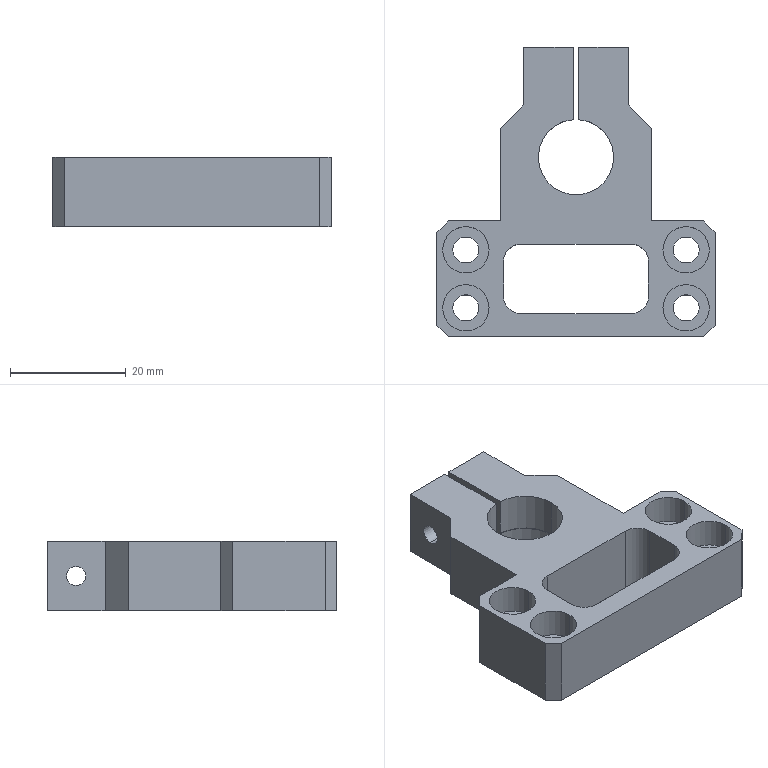Part | SolidWorks | features ICE 5, Chamfer 3, HoleWzd 3, Cut 1, Extrusion 1, Fillet 1 | 1 solid | 63 faces | box 48 x 50 x 12 mm | volume 12507 mm3 | cylinder 30 | plane 30 | cone 3 | commonest cylinder face diameters 4.5 x10 8 x8 6 x4 13 x3 15 x3 3.3 x2